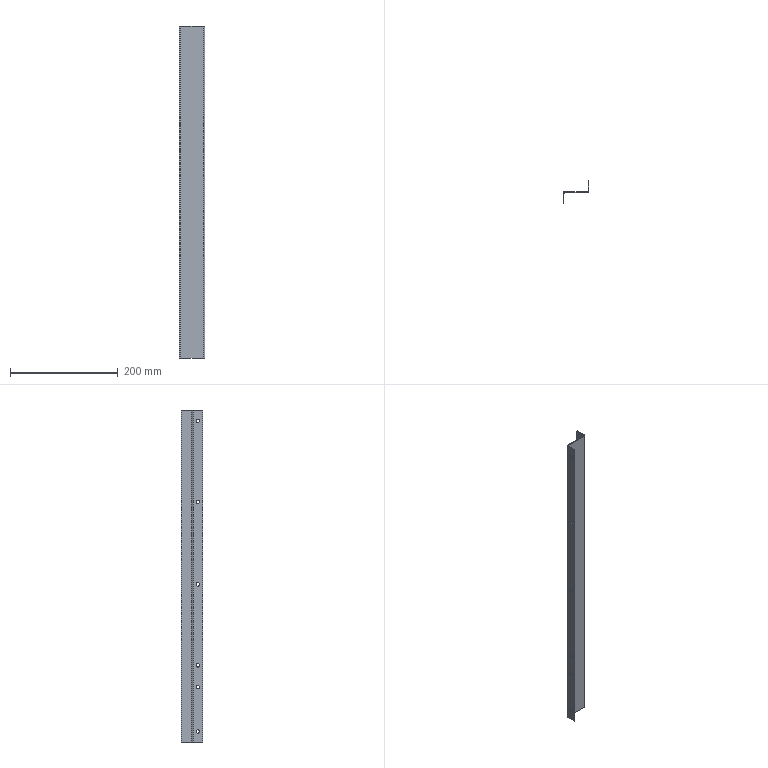Part | SolidWorks | features Cut 1, FlatPattern 1, SMBaseFlange 1, SheetMetal 1 | 1 solid | 34 faces | box 47.2 x 40 x 615 mm | volume 62089 mm3 | plane 18 | cylinder 16 | commonest cylinder face diameters 6.5 x12 2.4 x2 4.8 x2
STEP:
#1=CARTESIAN_POINT('',(1.2,12.25,595.));
#2=VERTEX_POINT('',#1);
#3=CARTESIAN_POINT('',(1.2,5.75,595.));
#4=VERTEX_POINT('',#3);
#5=CARTESIAN_POINT('',(1.2,9.,595.));
#6=DIRECTION('',(-1.,0.,0.));
#7=DIRECTION('',(0.,0.,1.));
#8=AXIS2_PLACEMENT_3D('',#5,#6,#7);
#9=CIRCLE('',#8,3.25);
#10=EDGE_CURVE('',#2,#4,#9,.T.);
#11=ORIENTED_EDGE('',*,*,#10,.F.);
#12=CARTESIAN_POINT('',(0.,12.25,595.));
#13=VERTEX_POINT('',#12);
#14=CARTESIAN_POINT('',(9.2,12.25,595.));
#15=DIRECTION('',(-1.,0.,0.));
#16=VECTOR('',#15,1000.);
#17=LINE('',#14,#16);
#18=EDGE_CURVE('',#2,#13,#17,.T.);
#19=ORIENTED_EDGE('',*,*,#18,.T.);
#20=CARTESIAN_POINT('',(0.,5.75,595.));
#21=VERTEX_POINT('',#20);
#22=CARTESIAN_POINT('',(0.,9.,595.));
#23=DIRECTION('',(-1.,0.,0.));
#24=DIRECTION('',(0.,0.,1.));
#25=AXIS2_PLACEMENT_3D('',#22,#23,#24);
#26=CIRCLE('',#25,3.25);
#27=EDGE_CURVE('',#13,#21,#26,.T.);
#28=ORIENTED_EDGE('',*,*,#27,.T.);
#29=CARTESIAN_POINT('',(9.2,5.75,595.));
#30=DIRECTION('',(-1.,0.,0.));
#31=VECTOR('',#30,1000.);
#32=LINE('',#29,#31);
#33=EDGE_CURVE('',#4,#21,#32,.T.);
#34=ORIENTED_EDGE('',*,*,#33,.F.);
#35=EDGE_LOOP('',(#11,#19,#28,#34));
#36=FACE_OUTER_BOUND('',#35,.T.);
#37=CARTESIAN_POINT('',(9.2,9.,595.));
#38=DIRECTION('',(-1.,0.,0.));
#39=DIRECTION('',(0.,-1.,0.));
#40=AXIS2_PLACEMENT_3D('',#37,#38,#39);
#41=CYLINDRICAL_SURFACE('',#40,3.25);
#42=ADVANCED_FACE('',(#36),#41,.F.);
#43=CARTESIAN_POINT('',(1.2,12.25,292.));
#44=VERTEX_POINT('',#43);
#45=CARTESIAN_POINT('',(1.2,5.75,292.));
#46=VERTEX_POINT('',#45);
#47=CARTESIAN_POINT('',(1.2,9.,292.));
#48=DIRECTION('',(-1.,0.,0.));
#49=DIRECTION('',(0.,0.,1.));
#50=AXIS2_PLACEMENT_3D('',#47,#48,#49);
#51=CIRCLE('',#50,3.25);
#52=EDGE_CURVE('',#44,#46,#51,.T.);
#53=ORIENTED_EDGE('',*,*,#52,.F.);
#54=CARTESIAN_POINT('',(0.,12.25,292.));
#55=VERTEX_POINT('',#54);
#56=CARTESIAN_POINT('',(9.2,12.25,292.));
#57=DIRECTION('',(-1.,0.,0.));
#58=VECTOR('',#57,1000.);
#59=LINE('',#56,#58);
#60=EDGE_CURVE('',#44,#55,#59,.T.);
#61=ORIENTED_EDGE('',*,*,#60,.T.);
#62=CARTESIAN_POINT('',(0.,5.75,292.));
#63=VERTEX_POINT('',#62);
#64=CARTESIAN_POINT('',(0.,9.,292.));
#65=DIRECTION('',(-1.,0.,0.));
#66=DIRECTION('',(0.,0.,1.));
#67=AXIS2_PLACEMENT_3D('',#64,#65,#66);
#68=CIRCLE('',#67,3.25);
#69=EDGE_CURVE('',#55,#63,#68,.T.);
#70=ORIENTED_EDGE('',*,*,#69,.T.);
#71=CARTESIAN_POINT('',(9.2,5.75,292.));
#72=DIRECTION('',(-1.,0.,0.));
#73=VECTOR('',#72,1000.);
#74=LINE('',#71,#73);
#75=EDGE_CURVE('',#46,#63,#74,.T.);
#76=ORIENTED_EDGE('',*,*,#75,.F.);
#77=EDGE_LOOP('',(#53,#61,#70,#76));
#78=FACE_OUTER_BOUND('',#77,.T.);
#79=CARTESIAN_POINT('',(9.2,9.,292.));
#80=DIRECTION('',(-1.,0.,0.));
#81=DIRECTION('',(0.,-1.,0.));
#82=AXIS2_PLACEMENT_3D('',#79,#80,#81);
#83=CYLINDRICAL_SURFACE('',#82,3.25);
#84=ADVANCED_FACE('',(#78),#83,.F.);
#85=CARTESIAN_POINT('',(1.2,12.25,445.));
#86=VERTEX_POINT('',#85);
#87=CARTESIAN_POINT('',(1.2,5.75,445.));
#88=VERTEX_POINT('',#87);
#89=CARTESIAN_POINT('',(1.2,9.,445.));
#90=DIRECTION('',(-1.,0.,0.));
#91=DIRECTION('',(0.,0.,1.));
#92=AXIS2_PLACEMENT_3D('',#89,#90,#91);
#93=CIRCLE('',#92,3.25);
#94=EDGE_CURVE('',#86,#88,#93,.T.);
#95=ORIENTED_EDGE('',*,*,#94,.F.);
#96=CARTESIAN_POINT('',(0.,12.25,445.));
#97=VERTEX_POINT('',#96);
#98=CARTESIAN_POINT('',(9.2,12.25,445.));
#99=DIRECTION('',(-1.,0.,0.));
#100=VECTOR('',#99,1000.);
#101=LINE('',#98,#100);
#102=EDGE_CURVE('',#86,#97,#101,.T.);
#103=ORIENTED_EDGE('',*,*,#102,.T.);
#104=CARTESIAN_POINT('',(0.,5.75,445.));
#105=VERTEX_POINT('',#104);
#106=CARTESIAN_POINT('',(0.,9.,445.));
#107=DIRECTION('',(-1.,0.,0.));
#108=DIRECTION('',(0.,0.,1.));
#109=AXIS2_PLACEMENT_3D('',#106,#107,#108);
#110=CIRCLE('',#109,3.25);
#111=EDGE_CURVE('',#97,#105,#110,.T.);
#112=ORIENTED_EDGE('',*,*,#111,.T.);
#113=CARTESIAN_POINT('',(9.2,5.75,445.));
#114=DIRECTION('',(-1.,0.,0.));
#115=VECTOR('',#114,1000.);
#116=LINE('',#113,#115);
#117=EDGE_CURVE('',#88,#105,#116,.T.);
#118=ORIENTED_EDGE('',*,*,#117,.F.);
#119=EDGE_LOOP('',(#95,#103,#112,#118));
#120=FACE_OUTER_BOUND('',#119,.T.);
#121=CARTESIAN_POINT('',(9.2,9.,445.));
#122=DIRECTION('',(-1.,0.,0.));
#123=DIRECTION('',(0.,-1.,0.));
#124=AXIS2_PLACEMENT_3D('',#121,#122,#123);
#125=CYLINDRICAL_SURFACE('',#124,3.25);
#126=ADVANCED_FACE('',(#120),#125,.F.);
#127=CARTESIAN_POINT('',(1.2,12.25,101.5));
#128=VERTEX_POINT('',#127);
#129=CARTESIAN_POINT('',(1.2,5.75,101.5));
#130=VERTEX_POINT('',#129);
#131=CARTESIAN_POINT('',(1.2,9.,101.5));
#132=DIRECTION('',(-1.,0.,0.));
#133=DIRECTION('',(0.,0.,1.));
#134=AXIS2_PLACEMENT_3D('',#131,#132,#133);
#135=CIRCLE('',#134,3.25);
#136=EDGE_CURVE('',#128,#130,#135,.T.);
#137=ORIENTED_EDGE('',*,*,#136,.F.);
#138=CARTESIAN_POINT('',(0.,12.25,101.5));
#139=VERTEX_POINT('',#138);
#140=CARTESIAN_POINT('',(9.2,12.25,101.5));
#141=DIRECTION('',(-1.,0.,0.));
#142=VECTOR('',#141,1000.);
#143=LINE('',#140,#142);
#144=EDGE_CURVE('',#128,#139,#143,.T.);
#145=ORIENTED_EDGE('',*,*,#144,.T.);
#146=CARTESIAN_POINT('',(0.,5.75,101.5));
#147=VERTEX_POINT('',#146);
#148=CARTESIAN_POINT('',(0.,9.,101.5));
#149=DIRECTION('',(-1.,0.,0.));
#150=DIRECTION('',(0.,0.,1.));
#151=AXIS2_PLACEMENT_3D('',#148,#149,#150);
#152=CIRCLE('',#151,3.25);
#153=EDGE_CURVE('',#139,#147,#152,.T.);
#154=ORIENTED_EDGE('',*,*,#153,.T.);
#155=CARTESIAN_POINT('',(9.2,5.75,101.5));
#156=DIRECTION('',(-1.,0.,0.));
#157=VECTOR('',#156,1000.);
#158=LINE('',#155,#157);
#159=EDGE_CURVE('',#130,#147,#158,.T.);
#160=ORIENTED_EDGE('',*,*,#159,.F.);
#161=EDGE_LOOP('',(#137,#145,#154,#160));
#162=FACE_OUTER_BOUND('',#161,.T.);
#163=CARTESIAN_POINT('',(9.2,9.,101.5));
#164=DIRECTION('',(-1.,0.,0.));
#165=DIRECTION('',(0.,-1.,0.));
#166=AXIS2_PLACEMENT_3D('',#163,#164,#165);
#167=CYLINDRICAL_SURFACE('',#166,3.25);
#168=ADVANCED_FACE('',(#162),#167,.F.);
#169=CARTESIAN_POINT('',(1.2,12.25,19.5));
#170=VERTEX_POINT('',#169);
#171=CARTESIAN_POINT('',(1.2,5.75,19.5));
#172=VERTEX_POINT('',#171);
#173=CARTESIAN_POINT('',(1.2,9.,19.5));
#174=DIRECTION('',(-1.,0.,0.));
#175=DIRECTION('',(0.,0.,1.));
#176=AXIS2_PLACEMENT_3D('',#173,#174,#175);
#177=CIRCLE('',#176,3.25);
#178=EDGE_CURVE('',#170,#172,#177,.T.);
#179=ORIENTED_EDGE('',*,*,#178,.F.);
#180=CARTESIAN_POINT('',(0.,12.25,19.5));
#181=VERTEX_POINT('',#180);
#182=CARTESIAN_POINT('',(9.2,12.25,19.5));
#183=DIRECTION('',(-1.,0.,0.));
#184=VECTOR('',#183,1000.);
#185=LINE('',#182,#184);
#186=EDGE_CURVE('',#170,#181,#185,.T.);
#187=ORIENTED_EDGE('',*,*,#186,.T.);
#188=CARTESIAN_POINT('',(0.,5.75,19.5));
#189=VERTEX_POINT('',#188);
#190=CARTESIAN_POINT('',(0.,9.,19.5));
#191=DIRECTION('',(-1.,0.,0.));
#192=DIRECTION('',(0.,0.,1.));
#193=AXIS2_PLACEMENT_3D('',#190,#191,#192);
#194=CIRCLE('',#193,3.25);
#195=EDGE_CURVE('',#181,#189,#194,.T.);
#196=ORIENTED_EDGE('',*,*,#195,.T.);
#197=CARTESIAN_POINT('',(9.2,5.75,19.5));
#198=DIRECTION('',(-1.,0.,0.));
#199=VECTOR('',#198,1000.);
#200=LINE('',#197,#199);
#201=EDGE_CURVE('',#172,#189,#200,.T.);
#202=ORIENTED_EDGE('',*,*,#201,.F.);
#203=EDGE_LOOP('',(#179,#187,#196,#202));
#204=FACE_OUTER_BOUND('',#203,.T.);
#205=CARTESIAN_POINT('',(9.2,9.,19.5));
#206=DIRECTION('',(-1.,0.,0.));
#207=DIRECTION('',(0.,-1.,0.));
#208=AXIS2_PLACEMENT_3D('',#205,#206,#207);
#209=CYLINDRICAL_SURFACE('',#208,3.25);
#210=ADVANCED_FACE('',(#204),#209,.F.);
#211=CARTESIAN_POINT('',(1.2,12.25,142.));
#212=VERTEX_POINT('',#211);
#213=CARTESIAN_POINT('',(1.2,5.75,142.));
#214=VERTEX_POINT('',#213);
#215=CARTESIAN_POINT('',(1.2,9.,142.));
#216=DIRECTION('',(-1.,0.,0.));
#217=DIRECTION('',(0.,0.,1.));
#218=AXIS2_PLACEMENT_3D('',#215,#216,#217);
#219=CIRCLE('',#218,3.25);
#220=EDGE_CURVE('',#212,#214,#219,.T.);
#221=ORIENTED_EDGE('',*,*,#220,.F.);
#222=CARTESIAN_POINT('',(0.,12.25,142.));
#223=VERTEX_POINT('',#222);
#224=CARTESIAN_POINT('',(9.2,12.25,142.));
#225=DIRECTION('',(-1.,0.,0.));
#226=VECTOR('',#225,1000.);
#227=LINE('',#224,#226);
#228=EDGE_CURVE('',#212,#223,#227,.T.);
#229=ORIENTED_EDGE('',*,*,#228,.T.);
#230=CARTESIAN_POINT('',(0.,5.75,142.));
#231=VERTEX_POINT('',#230);
#232=CARTESIAN_POINT('',(0.,9.,142.));
#233=DIRECTION('',(-1.,0.,0.));
#234=DIRECTION('',(0.,0.,1.));
#235=AXIS2_PLACEMENT_3D('',#232,#233,#234);
#236=CIRCLE('',#235,3.25);
#237=EDGE_CURVE('',#223,#231,#236,.T.);
#238=ORIENTED_EDGE('',*,*,#237,.T.);
#239=CARTESIAN_POINT('',(9.2,5.75,142.));
#240=DIRECTION('',(-1.,0.,0.));
#241=VECTOR('',#240,1000.);
#242=LINE('',#239,#241);
#243=EDGE_CURVE('',#214,#231,#242,.T.);
#244=ORIENTED_EDGE('',*,*,#243,.F.);
#245=EDGE_LOOP('',(#221,#229,#238,#244));
#246=FACE_OUTER_BOUND('',#245,.T.);
#247=CARTESIAN_POINT('',(9.2,9.,142.));
#248=DIRECTION('',(-1.,0.,0.));
#249=DIRECTION('',(0.,-1.,0.));
#250=AXIS2_PLACEMENT_3D('',#247,#248,#249);
#251=CYLINDRICAL_SURFACE('',#250,3.25);
#252=ADVANCED_FACE('',(#246),#251,.F.);
#253=CARTESIAN_POINT('',(2.4,20.,615.));
#254=VERTEX_POINT('',#253);
#255=CARTESIAN_POINT('',(2.4,18.8,615.));
#256=VERTEX_POINT('',#255);
#257=CARTESIAN_POINT('',(2.4,20.,615.));
#258=DIRECTION('',(0.,-1.,0.));
#259=VECTOR('',#258,1000.);
#260=LINE('',#257,#259);
#261=EDGE_CURVE('',#254,#256,#260,.T.);
#262=ORIENTED_EDGE('',*,*,#261,.F.);
#263=CARTESIAN_POINT('',(0.,17.6,615.));
#264=VERTEX_POINT('',#263);
#265=CARTESIAN_POINT('',(2.4,17.6,615.));
#266=DIRECTION('',(0.,0.,-1.));
#267=DIRECTION('',(1.,0.,0.));
#268=AXIS2_PLACEMENT_3D('',#265,#266,#267);
#269=CIRCLE('',#268,2.4);
#270=EDGE_CURVE('',#264,#254,#269,.T.);
#271=ORIENTED_EDGE('',*,*,#270,.F.);
#272=CARTESIAN_POINT('',(1.2,17.6,615.));
#273=VERTEX_POINT('',#272);
#274=CARTESIAN_POINT('',(1.2,17.6,615.));
#275=DIRECTION('',(-1.,0.,0.));
#276=VECTOR('',#275,1000.);
#277=LINE('',#274,#276);
#278=EDGE_CURVE('',#273,#264,#277,.T.);
#279=ORIENTED_EDGE('',*,*,#278,.F.);
#280=CARTESIAN_POINT('',(2.4,17.6,615.));
#281=DIRECTION('',(0.,0.,-1.));
#282=DIRECTION('',(1.,0.,0.));
#283=AXIS2_PLACEMENT_3D('',#280,#281,#282);
#284=CIRCLE('',#283,1.2);
#285=EDGE_CURVE('',#273,#256,#284,.T.);
#286=ORIENTED_EDGE('',*,*,#285,.T.);
#287=EDGE_LOOP('',(#262,#271,#279,#286));
#288=FACE_OUTER_BOUND('',#287,.T.);
#289=CARTESIAN_POINT('',(2.4,20.,615.));
#290=DIRECTION('',(0.,0.,1.));
#291=DIRECTION('',(1.,0.,0.));
#292=AXIS2_PLACEMENT_3D('',#289,#290,#291);
#293=PLANE('',#292);
#294=ADVANCED_FACE('',(#288),#293,.T.);
#295=CARTESIAN_POINT('',(44.8,20.,615.));
#296=VERTEX_POINT('',#295);
#297=CARTESIAN_POINT('',(0.,20.,615.));
#298=DIRECTION('',(1.,0.,0.));
#299=VECTOR('',#298,1000.);
#300=LINE('',#297,#299);
#301=EDGE_CURVE('',#254,#296,#300,.T.);
#302=ORIENTED_EDGE('',*,*,#301,.F.);
#303=ORIENTED_EDGE('',*,*,#261,.T.);
#304=CARTESIAN_POINT('',(44.8,18.8,615.));
#305=VERTEX_POINT('',#304);
#306=CARTESIAN_POINT('',(0.,18.8,615.));
#307=DIRECTION('',(1.,0.,0.));
#308=VECTOR('',#307,1000.);
#309=LINE('',#306,#308);
#310=EDGE_CURVE('',#256,#305,#309,.T.);
#311=ORIENTED_EDGE('',*,*,#310,.T.);
#312=CARTESIAN_POINT('',(44.8,18.8,615.));
#313=DIRECTION('',(0.,1.,0.));
#314=VECTOR('',#313,1000.);
#315=LINE('',#312,#314);
#316=EDGE_CURVE('',#305,#296,#315,.T.);
#317=ORIENTED_EDGE('',*,*,#316,.T.);
#318=EDGE_LOOP('',(#302,#303,#311,#317));
#319=FACE_OUTER_BOUND('',#318,.T.);
#320=CARTESIAN_POINT('',(1.2,17.6,615.));
#321=DIRECTION('',(0.,0.,1.));
#322=DIRECTION('',(1.,0.,0.));
#323=AXIS2_PLACEMENT_3D('',#320,#321,#322);
#324=PLANE('',#323);
#325=ADVANCED_FACE('',(#319),#324,.T.);
#326=CARTESIAN_POINT('',(0.,17.6,0.));
#327=VERTEX_POINT('',#326);
#328=CARTESIAN_POINT('',(1.2,17.6,0.));
#329=VERTEX_POINT('',#328);
#330=CARTESIAN_POINT('',(0.,17.6,0.));
#331=DIRECTION('',(1.,0.,0.));
#332=VECTOR('',#331,1000.);
#333=LINE('',#330,#332);
#334=EDGE_CURVE('',#327,#329,#333,.T.);
#335=ORIENTED_EDGE('',*,*,#334,.F.);
#336=CARTESIAN_POINT('',(2.4,20.,0.));
#337=VERTEX_POINT('',#336);
#338=CARTESIAN_POINT('',(2.4,17.6,0.));
#339=DIRECTION('',(0.,0.,-1.));
#340=DIRECTION('',(1.,0.,0.));
#341=AXIS2_PLACEMENT_3D('',#338,#339,#340);
#342=CIRCLE('',#341,2.4);
#343=EDGE_CURVE('',#327,#337,#342,.T.);
#344=ORIENTED_EDGE('',*,*,#343,.T.);
#345=CARTESIAN_POINT('',(2.4,18.8,0.));
#346=VERTEX_POINT('',#345);
#347=CARTESIAN_POINT('',(2.4,18.8,0.));
#348=DIRECTION('',(0.,1.,0.));
#349=VECTOR('',#348,1000.);
#350=LINE('',#347,#349);
#351=EDGE_CURVE('',#346,#337,#350,.T.);
#352=ORIENTED_EDGE('',*,*,#351,.F.);
#353=CARTESIAN_POINT('',(2.4,17.6,0.));
#354=DIRECTION('',(0.,0.,-1.));
#355=DIRECTION('',(1.,0.,0.));
#356=AXIS2_PLACEMENT_3D('',#353,#354,#355);
#357=CIRCLE('',#356,1.2);
#358=EDGE_CURVE('',#329,#346,#357,.T.);
#359=ORIENTED_EDGE('',*,*,#358,.F.);
#360=EDGE_LOOP('',(#335,#344,#352,#359));
#361=FACE_OUTER_BOUND('',#360,.T.);
#362=CARTESIAN_POINT('',(0.,17.6,0.));
#363=DIRECTION('',(0.,0.,-1.));
#364=DIRECTION('',(-1.,0.,0.));
#365=AXIS2_PLACEMENT_3D('',#362,#363,#364);
#366=PLANE('',#365);
#367=ADVANCED_FACE('',(#361),#366,.T.);
#368=CARTESIAN_POINT('',(0.,0.,0.));
#369=VERTEX_POINT('',#368);
#370=CARTESIAN_POINT('',(0.,0.,0.));
#371=DIRECTION('',(0.,1.,0.));
#372=VECTOR('',#371,1000.);
#373=LINE('',#370,#372);
#374=EDGE_CURVE('',#369,#327,#373,.T.);
#375=ORIENTED_EDGE('',*,*,#374,.T.);
#376=ORIENTED_EDGE('',*,*,#334,.T.);
#377=CARTESIAN_POINT('',(1.2,0.,0.));
#378=VERTEX_POINT('',#377);
#379=CARTESIAN_POINT('',(1.2,0.,0.));
#380=DIRECTION('',(0.,1.,0.));
#381=VECTOR('',#380,1000.);
#382=LINE('',#379,#381);
#383=EDGE_CURVE('',#378,#329,#382,.T.);
#384=ORIENTED_EDGE('',*,*,#383,.F.);
#385=CARTESIAN_POINT('',(1.2,0.,0.));
#386=DIRECTION('',(-1.,0.,0.));
#387=VECTOR('',#386,1000.);
#388=LINE('',#385,#387);
#389=EDGE_CURVE('',#378,#369,#388,.T.);
#390=ORIENTED_EDGE('',*,*,#389,.T.);
#391=EDGE_LOOP('',(#375,#376,#384,#390));
#392=FACE_OUTER_BOUND('',#391,.T.);
#393=CARTESIAN_POINT('',(2.4,18.8,0.));
#394=DIRECTION('',(0.,0.,-1.));
#395=DIRECTION('',(-1.,0.,0.));
#396=AXIS2_PLACEMENT_3D('',#393,#394,#395);
#397=PLANE('',#396);
#398=ADVANCED_FACE('',(#392),#397,.T.);
#399=CARTESIAN_POINT('',(46.,21.2,615.));
#400=VERTEX_POINT('',#399);
#401=CARTESIAN_POINT('',(47.2,21.2,615.));
#402=VERTEX_POINT('',#401);
#403=CARTESIAN_POINT('',(46.,21.2,615.));
#404=DIRECTION('',(1.,0.,0.));
#405=VECTOR('',#404,1000.);
#406=LINE('',#403,#405);
#407=EDGE_CURVE('',#400,#402,#406,.T.);
#408=ORIENTED_EDGE('',*,*,#407,.F.);
#409=CARTESIAN_POINT('',(44.8,21.2,615.));
#410=DIRECTION('',(0.,0.,1.));
#411=DIRECTION('',(-1.,0.,0.));
#412=AXIS2_PLACEMENT_3D('',#409,#410,#411);
#413=CIRCLE('',#412,1.2);
#414=EDGE_CURVE('',#296,#400,#413,.T.);
#415=ORIENTED_EDGE('',*,*,#414,.F.);
#416=ORIENTED_EDGE('',*,*,#316,.F.);
#417=CARTESIAN_POINT('',(44.8,21.2,615.));
#418=DIRECTION('',(0.,0.,1.));
#419=DIRECTION('',(1.,0.,0.));
#420=AXIS2_PLACEMENT_3D('',#417,#418,#419);
#421=CIRCLE('',#420,2.4);
#422=EDGE_CURVE('',#305,#402,#421,.T.);
#423=ORIENTED_EDGE('',*,*,#422,.T.);
#424=EDGE_LOOP('',(#408,#415,#416,#423));
#425=FACE_OUTER_BOUND('',#424,.T.);
#426=CARTESIAN_POINT('',(46.,21.2,615.));
#427=DIRECTION('',(0.,0.,1.));
#428=DIRECTION('',(1.,0.,0.));
#429=AXIS2_PLACEMENT_3D('',#426,#427,#428);
#430=PLANE('',#429);
#431=ADVANCED_FACE('',(#425),#430,.T.);
#432=CARTESIAN_POINT('',(46.,40.,615.));
#433=VERTEX_POINT('',#432);
#434=CARTESIAN_POINT('',(46.,20.,615.));
#435=DIRECTION('',(0.,1.,0.));
#436=VECTOR('',#435,1000.);
#437=LINE('',#434,#436);
#438=EDGE_CURVE('',#400,#433,#437,.T.);
#439=ORIENTED_EDGE('',*,*,#438,.F.);
#440=ORIENTED_EDGE('',*,*,#407,.T.);
#441=CARTESIAN_POINT('',(47.2,40.,615.));
#442=VERTEX_POINT('',#441);
#443=CARTESIAN_POINT('',(47.2,20.,615.));
#444=DIRECTION('',(0.,1.,0.));
#445=VECTOR('',#444,1000.);
#446=LINE('',#443,#445);
#447=EDGE_CURVE('',#402,#442,#446,.T.);
#448=ORIENTED_EDGE('',*,*,#447,.T.);
#449=CARTESIAN_POINT('',(46.,40.,615.));
#450=DIRECTION('',(1.,0.,0.));
#451=VECTOR('',#450,1000.);
#452=LINE('',#449,#451);
#453=EDGE_CURVE('',#433,#442,#452,.T.);
#454=ORIENTED_EDGE('',*,*,#453,.F.);
#455=EDGE_LOOP('',(#439,#440,#448,#454));
#456=FACE_OUTER_BOUND('',#455,.T.);
#457=CARTESIAN_POINT('',(44.8,18.8,615.));
#458=DIRECTION('',(0.,0.,1.));
#459=DIRECTION('',(1.,0.,0.));
#460=AXIS2_PLACEMENT_3D('',#457,#458,#459);
#461=PLANE('',#460);
#462=ADVANCED_FACE('',(#456),#461,.T.);
#463=CARTESIAN_POINT('',(44.8,20.,0.));
#464=VERTEX_POINT('',#463);
#465=CARTESIAN_POINT('',(44.8,18.8,0.));
#466=VERTEX_POINT('',#465);
#467=CARTESIAN_POINT('',(44.8,20.,0.));
#468=DIRECTION('',(0.,-1.,0.));
#469=VECTOR('',#468,1000.);
#470=LINE('',#467,#469);
#471=EDGE_CURVE('',#464,#466,#470,.T.);
#472=ORIENTED_EDGE('',*,*,#471,.F.);
#473=CARTESIAN_POINT('',(46.,21.2,0.));
#474=VERTEX_POINT('',#473);
#475=CARTESIAN_POINT('',(44.8,21.2,0.));
#476=DIRECTION('',(0.,0.,1.));
#477=DIRECTION('',(-1.,0.,0.));
#478=AXIS2_PLACEMENT_3D('',#475,#476,#477);
#479=CIRCLE('',#478,1.2);
#480=EDGE_CURVE('',#464,#474,#479,.T.);
#481=ORIENTED_EDGE('',*,*,#480,.T.);
#482=CARTESIAN_POINT('',(47.2,21.2,0.));
#483=VERTEX_POINT('',#482);
#484=CARTESIAN_POINT('',(47.2,21.2,0.));
#485=DIRECTION('',(-1.,0.,0.));
#486=VECTOR('',#485,1000.);
#487=LINE('',#484,#486);
#488=EDGE_CURVE('',#483,#474,#487,.T.);
#489=ORIENTED_EDGE('',*,*,#488,.F.);
#490=CARTESIAN_POINT('',(44.8,21.2,0.));
#491=DIRECTION('',(0.,0.,1.));
#492=DIRECTION('',(1.,0.,0.));
#493=AXIS2_PLACEMENT_3D('',#490,#491,#492);
#494=CIRCLE('',#493,2.4);
#495=EDGE_CURVE('',#466,#483,#494,.T.);
#496=ORIENTED_EDGE('',*,*,#495,.F.);
#497=EDGE_LOOP('',(#472,#481,#489,#496));
#498=FACE_OUTER_BOUND('',#497,.T.);
#499=CARTESIAN_POINT('',(44.8,20.,0.));
#500=DIRECTION('',(0.,0.,-1.));
#501=DIRECTION('',(-1.,0.,0.));
#502=AXIS2_PLACEMENT_3D('',#499,#500,#501);
#503=PLANE('',#502);
#504=ADVANCED_FACE('',(#498),#503,.T.);
#505=CARTESIAN_POINT('',(0.,20.,0.));
#506=DIRECTION('',(1.,0.,0.));
#507=VECTOR('',#506,1000.);
#508=LINE('',#505,#507);
#509=EDGE_CURVE('',#337,#464,#508,.T.);
#510=ORIENTED_EDGE('',*,*,#509,.T.);
#511=ORIENTED_EDGE('',*,*,#471,.T.);
#512=CARTESIAN_POINT('',(0.,18.8,0.));
#513=DIRECTION('',(1.,0.,0.));
#514=VECTOR('',#513,1000.);
#515=LINE('',#512,#514);
#516=EDGE_CURVE('',#346,#466,#515,.T.);
#517=ORIENTED_EDGE('',*,*,#516,.F.);
#518=ORIENTED_EDGE('',*,*,#351,.T.);
#519=EDGE_LOOP('',(#510,#511,#517,#518));
#520=FACE_OUTER_BOUND('',#519,.T.);
#521=CARTESIAN_POINT('',(47.2,21.2,0.));
#522=DIRECTION('',(0.,0.,-1.));
#523=DIRECTION('',(-1.,0.,0.));
#524=AXIS2_PLACEMENT_3D('',#521,#522,#523);
#525=PLANE('',#524);
#526=ADVANCED_FACE('',(#520),#525,.T.);
#527=CARTESIAN_POINT('',(47.2,40.,0.));
#528=VERTEX_POINT('',#527);
#529=CARTESIAN_POINT('',(47.2,20.,0.));
#530=DIRECTION('',(0.,1.,0.));
#531=VECTOR('',#530,1000.);
#532=LINE('',#529,#531);
#533=EDGE_CURVE('',#483,#528,#532,.T.);
#534=ORIENTED_EDGE('',*,*,#533,.T.);
#535=CARTESIAN_POINT('',(47.2,40.,615.));
#536=DIRECTION('',(0.,0.,-1.));
#537=VECTOR('',#536,1000.);
#538=LINE('',#535,#537);
#539=EDGE_CURVE('',#442,#528,#538,.T.);
#540=ORIENTED_EDGE('',*,*,#539,.F.);
#541=ORIENTED_EDGE('',*,*,#447,.F.);
#542=CARTESIAN_POINT('',(47.2,21.2,615.));
#543=DIRECTION('',(0.,0.,-1.));
#544=VECTOR('',#543,1000.);
#545=LINE('',#542,#544);
#546=EDGE_CURVE('',#402,#483,#545,.T.);
#547=ORIENTED_EDGE('',*,*,#546,.T.);
#548=EDGE_LOOP('',(#534,#540,#541,#547));
#549=FACE_OUTER_BOUND('',#548,.T.);
#550=CARTESIAN_POINT('',(47.2,20.,615.));
#551=DIRECTION('',(-1.,0.,0.));
#552=DIRECTION('',(0.,0.,1.));
#553=AXIS2_PLACEMENT_3D('',#550,#551,#552);
#554=PLANE('',#553);
#555=ADVANCED_FACE('',(#549),#554,.F.);
#556=CARTESIAN_POINT('',(46.,40.,0.));
#557=VERTEX_POINT('',#556);
#558=CARTESIAN_POINT('',(46.,40.,0.));
#559=DIRECTION('',(1.,0.,0.));
#560=VECTOR('',#559,1000.);
#561=LINE('',#558,#560);
#562=EDGE_CURVE('',#557,#528,#561,.T.);
#563=ORIENTED_EDGE('',*,*,#562,.F.);
#564=CARTESIAN_POINT('',(46.,40.,615.));
#565=DIRECTION('',(0.,0.,-1.));
#566=VECTOR('',#565,1000.);
#567=LINE('',#564,#566);
#568=EDGE_CURVE('',#433,#557,#567,.T.);
#569=ORIENTED_EDGE('',*,*,#568,.F.);
#570=ORIENTED_EDGE('',*,*,#453,.T.);
#571=ORIENTED_EDGE('',*,*,#539,.T.);
#572=EDGE_LOOP('',(#563,#569,#570,#571));
#573=FACE_OUTER_BOUND('',#572,.T.);
#574=CARTESIAN_POINT('',(46.,40.,615.));
#575=DIRECTION('',(0.,1.,0.));
#576=DIRECTION('',(0.,0.,1.));
#577=AXIS2_PLACEMENT_3D('',#574,#575,#576);
#578=PLANE('',#577);
#579=ADVANCED_FACE('',(#573),#578,.T.);
#580=CARTESIAN_POINT('',(46.,20.,0.));
#581=DIRECTION('',(0.,1.,0.));
#582=VECTOR('',#581,1000.);
#583=LINE('',#580,#582);
#584=EDGE_CURVE('',#474,#557,#583,.T.);
#585=ORIENTED_EDGE('',*,*,#584,.F.);
#586=CARTESIAN_POINT('',(46.,21.2,615.));
#587=DIRECTION('',(0.,0.,-1.));
#588=VECTOR('',#587,1000.);
#589=LINE('',#586,#588);
#590=EDGE_CURVE('',#400,#474,#589,.T.);
#591=ORIENTED_EDGE('',*,*,#590,.F.);
#592=ORIENTED_EDGE('',*,*,#438,.T.);
#593=ORIENTED_EDGE('',*,*,#568,.T.);
#594=EDGE_LOOP('',(#585,#591,#592,#593));
#595=FACE_OUTER_BOUND('',#594,.T.);
#596=CARTESIAN_POINT('',(46.,20.,615.));
#597=DIRECTION('',(-1.,0.,0.));
#598=DIRECTION('',(0.,0.,1.));
#599=AXIS2_PLACEMENT_3D('',#596,#597,#598);
#600=PLANE('',#599);
#601=ADVANCED_FACE('',(#595),#600,.T.);
#602=ORIENTED_EDGE('',*,*,#480,.F.);
#603=CARTESIAN_POINT('',(44.8,20.,615.));
#604=DIRECTION('',(0.,0.,-1.));
#605=VECTOR('',#604,1000.);
#606=LINE('',#603,#605);
#607=EDGE_CURVE('',#296,#464,#606,.T.);
#608=ORIENTED_EDGE('',*,*,#607,.F.);
#609=ORIENTED_EDGE('',*,*,#414,.T.);
#610=ORIENTED_EDGE('',*,*,#590,.T.);
#611=EDGE_LOOP('',(#602,#608,#609,#610));
#612=FACE_OUTER_BOUND('',#611,.T.);
#613=CARTESIAN_POINT('',(44.8,21.2,615.));
#614=DIRECTION('',(0.,0.,-1.));
#615=DIRECTION('',(-1.,0.,0.));
#616=AXIS2_PLACEMENT_3D('',#613,#614,#615);
#617=CYLINDRICAL_SURFACE('',#616,1.2);
#618=ADVANCED_FACE('',(#612),#617,.F.);
#619=ORIENTED_EDGE('',*,*,#509,.F.);
#620=CARTESIAN_POINT('',(2.4,20.,615.));
#621=DIRECTION('',(0.,0.,-1.));
#622=VECTOR('',#621,1000.);
#623=LINE('',#620,#622);
#624=EDGE_CURVE('',#254,#337,#623,.T.);
#625=ORIENTED_EDGE('',*,*,#624,.F.);
#626=ORIENTED_EDGE('',*,*,#301,.T.);
#627=ORIENTED_EDGE('',*,*,#607,.T.);
#628=EDGE_LOOP('',(#619,#625,#626,#627));
#629=FACE_OUTER_BOUND('',#628,.T.);
#630=CARTESIAN_POINT('',(0.,20.,615.));
#631=DIRECTION('',(0.,1.,0.));
#632=DIRECTION('',(0.,0.,1.));
#633=AXIS2_PLACEMENT_3D('',#630,#631,#632);
#634=PLANE('',#633);
#635=ADVANCED_FACE('',(#629),#634,.T.);
#636=ORIENTED_EDGE('',*,*,#343,.F.);
#637=CARTESIAN_POINT('',(0.,17.6,615.));
#638=DIRECTION('',(0.,0.,-1.));
#639=VECTOR('',#638,1000.);
#640=LINE('',#637,#639);
#641=EDGE_CURVE('',#264,#327,#640,.T.);
#642=ORIENTED_EDGE('',*,*,#641,.F.);
#643=ORIENTED_EDGE('',*,*,#270,.T.);
#644=ORIENTED_EDGE('',*,*,#624,.T.);
#645=EDGE_LOOP('',(#636,#642,#643,#644));
#646=FACE_OUTER_BOUND('',#645,.T.);
#647=CARTESIAN_POINT('',(2.4,17.6,615.));
#648=DIRECTION('',(0.,0.,-1.));
#649=DIRECTION('',(-1.,0.,0.));
#650=AXIS2_PLACEMENT_3D('',#647,#648,#649);
#651=CYLINDRICAL_SURFACE('',#650,2.4);
#652=ADVANCED_FACE('',(#646),#651,.T.);
#653=CARTESIAN_POINT('',(0.,9.,595.));
#654=DIRECTION('',(-1.,0.,0.));
#655=DIRECTION('',(0.,0.,1.));
#656=AXIS2_PLACEMENT_3D('',#653,#654,#655);
#657=CIRCLE('',#656,3.25);
#658=EDGE_CURVE('',#21,#13,#657,.T.);
#659=ORIENTED_EDGE('',*,*,#658,.F.);
#660=ORIENTED_EDGE('',*,*,#27,.F.);
#661=EDGE_LOOP('',(#659,#660));
#662=FACE_BOUND('',#661,.T.);
#663=CARTESIAN_POINT('',(0.,9.,292.));
#664=DIRECTION('',(-1.,0.,0.));
#665=DIRECTION('',(0.,0.,1.));
#666=AXIS2_PLACEMENT_3D('',#663,#664,#665);
#667=CIRCLE('',#666,3.25);
#668=EDGE_CURVE('',#63,#55,#667,.T.);
#669=ORIENTED_EDGE('',*,*,#668,.F.);
#670=ORIENTED_EDGE('',*,*,#69,.F.);
#671=EDGE_LOOP('',(#669,#670));
#672=FACE_BOUND('',#671,.T.);
#673=CARTESIAN_POINT('',(0.,9.,445.));
#674=DIRECTION('',(-1.,0.,0.));
#675=DIRECTION('',(0.,0.,1.));
#676=AXIS2_PLACEMENT_3D('',#673,#674,#675);
#677=CIRCLE('',#676,3.25);
#678=EDGE_CURVE('',#105,#97,#677,.T.);
#679=ORIENTED_EDGE('',*,*,#678,.F.);
#680=ORIENTED_EDGE('',*,*,#111,.F.);
#681=EDGE_LOOP('',(#679,#680));
#682=FACE_BOUND('',#681,.T.);
#683=CARTESIAN_POINT('',(0.,9.,101.5));
#684=DIRECTION('',(-1.,0.,0.));
#685=DIRECTION('',(0.,0.,1.));
#686=AXIS2_PLACEMENT_3D('',#683,#684,#685);
#687=CIRCLE('',#686,3.25);
#688=EDGE_CURVE('',#147,#139,#687,.T.);
#689=ORIENTED_EDGE('',*,*,#688,.F.);
#690=ORIENTED_EDGE('',*,*,#153,.F.);
#691=EDGE_LOOP('',(#689,#690));
#692=FACE_BOUND('',#691,.T.);
#693=CARTESIAN_POINT('',(0.,9.,19.5));
#694=DIRECTION('',(-1.,0.,0.));
#695=DIRECTION('',(0.,0.,1.));
#696=AXIS2_PLACEMENT_3D('',#693,#694,#695);
#697=CIRCLE('',#696,3.25);
#698=EDGE_CURVE('',#189,#181,#697,.T.);
#699=ORIENTED_EDGE('',*,*,#698,.F.);
#700=ORIENTED_EDGE('',*,*,#195,.F.);
#701=EDGE_LOOP('',(#699,#700));
#702=FACE_BOUND('',#701,.T.);
#703=CARTESIAN_POINT('',(0.,9.,142.));
#704=DIRECTION('',(-1.,0.,0.));
#705=DIRECTION('',(0.,0.,1.));
#706=AXIS2_PLACEMENT_3D('',#703,#704,#705);
#707=CIRCLE('',#706,3.25);
#708=EDGE_CURVE('',#231,#223,#707,.T.);
#709=ORIENTED_EDGE('',*,*,#708,.F.);
#710=ORIENTED_EDGE('',*,*,#237,.F.);
#711=EDGE_LOOP('',(#709,#710));
#712=FACE_BOUND('',#711,.T.);
#713=ORIENTED_EDGE('',*,*,#374,.F.);
#714=CARTESIAN_POINT('',(0.,0.,615.));
#715=VERTEX_POINT('',#714);
#716=CARTESIAN_POINT('',(0.,0.,615.));
#717=DIRECTION('',(0.,0.,-1.));
#718=VECTOR('',#717,1000.);
#719=LINE('',#716,#718);
#720=EDGE_CURVE('',#715,#369,#719,.T.);
#721=ORIENTED_EDGE('',*,*,#720,.F.);
#722=CARTESIAN_POINT('',(0.,0.,615.));
#723=DIRECTION('',(0.,1.,0.));
#724=VECTOR('',#723,1000.);
#725=LINE('',#722,#724);
#726=EDGE_CURVE('',#715,#264,#725,.T.);
#727=ORIENTED_EDGE('',*,*,#726,.T.);
#728=ORIENTED_EDGE('',*,*,#641,.T.);
#729=EDGE_LOOP('',(#713,#721,#727,#728));
#730=FACE_OUTER_BOUND('',#729,.T.);
#731=CARTESIAN_POINT('',(0.,0.,615.));
#732=DIRECTION('',(-1.,0.,0.));
#733=DIRECTION('',(0.,0.,1.));
#734=AXIS2_PLACEMENT_3D('',#731,#732,#733);
#735=PLANE('',#734);
#736=ADVANCED_FACE('',(#662,#672,#682,#692,#702,#712,#730),#735,.T.);
#737=ORIENTED_EDGE('',*,*,#389,.F.);
#738=CARTESIAN_POINT('',(1.2,0.,615.));
#739=VERTEX_POINT('',#738);
#740=CARTESIAN_POINT('',(1.2,0.,615.));
#741=DIRECTION('',(0.,0.,-1.));
#742=VECTOR('',#741,1000.);
#743=LINE('',#740,#742);
#744=EDGE_CURVE('',#739,#378,#743,.T.);
#745=ORIENTED_EDGE('',*,*,#744,.F.);
#746=CARTESIAN_POINT('',(1.2,0.,615.));
#747=DIRECTION('',(-1.,0.,0.));
#748=VECTOR('',#747,1000.);
#749=LINE('',#746,#748);
#750=EDGE_CURVE('',#739,#715,#749,.T.);
#751=ORIENTED_EDGE('',*,*,#750,.T.);
#752=ORIENTED_EDGE('',*,*,#720,.T.);
#753=EDGE_LOOP('',(#737,#745,#751,#752));
#754=FACE_OUTER_BOUND('',#753,.T.);
#755=CARTESIAN_POINT('',(1.2,0.,615.));
#756=DIRECTION('',(0.,-1.,0.));
#757=DIRECTION('',(0.,0.,-1.));
#758=AXIS2_PLACEMENT_3D('',#755,#756,#757);
#759=PLANE('',#758);
#760=ADVANCED_FACE('',(#754),#759,.T.);
#761=CARTESIAN_POINT('',(1.2,9.,595.));
#762=DIRECTION('',(-1.,0.,0.));
#763=DIRECTION('',(0.,0.,1.));
#764=AXIS2_PLACEMENT_3D('',#761,#762,#763);
#765=CIRCLE('',#764,3.25);
#766=EDGE_CURVE('',#4,#2,#765,.T.);
#767=ORIENTED_EDGE('',*,*,#766,.T.);
#768=ORIENTED_EDGE('',*,*,#10,.T.);
#769=EDGE_LOOP('',(#767,#768));
#770=FACE_BOUND('',#769,.T.);
#771=CARTESIAN_POINT('',(1.2,9.,292.));
#772=DIRECTION('',(-1.,0.,0.));
#773=DIRECTION('',(0.,0.,1.));
#774=AXIS2_PLACEMENT_3D('',#771,#772,#773);
#775=CIRCLE('',#774,3.25);
#776=EDGE_CURVE('',#46,#44,#775,.T.);
#777=ORIENTED_EDGE('',*,*,#776,.T.);
#778=ORIENTED_EDGE('',*,*,#52,.T.);
#779=EDGE_LOOP('',(#777,#778));
#780=FACE_BOUND('',#779,.T.);
#781=CARTESIAN_POINT('',(1.2,9.,445.));
#782=DIRECTION('',(-1.,0.,0.));
#783=DIRECTION('',(0.,0.,1.));
#784=AXIS2_PLACEMENT_3D('',#781,#782,#783);
#785=CIRCLE('',#784,3.25);
#786=EDGE_CURVE('',#88,#86,#785,.T.);
#787=ORIENTED_EDGE('',*,*,#786,.T.);
#788=ORIENTED_EDGE('',*,*,#94,.T.);
#789=EDGE_LOOP('',(#787,#788));
#790=FACE_BOUND('',#789,.T.);
#791=CARTESIAN_POINT('',(1.2,9.,101.5));
#792=DIRECTION('',(-1.,0.,0.));
#793=DIRECTION('',(0.,0.,1.));
#794=AXIS2_PLACEMENT_3D('',#791,#792,#793);
#795=CIRCLE('',#794,3.25);
#796=EDGE_CURVE('',#130,#128,#795,.T.);
#797=ORIENTED_EDGE('',*,*,#796,.T.);
#798=ORIENTED_EDGE('',*,*,#136,.T.);
#799=EDGE_LOOP('',(#797,#798));
#800=FACE_BOUND('',#799,.T.);
#801=CARTESIAN_POINT('',(1.2,9.,19.5));
#802=DIRECTION('',(-1.,0.,0.));
#803=DIRECTION('',(0.,0.,1.));
#804=AXIS2_PLACEMENT_3D('',#801,#802,#803);
#805=CIRCLE('',#804,3.25);
#806=EDGE_CURVE('',#172,#170,#805,.T.);
#807=ORIENTED_EDGE('',*,*,#806,.T.);
#808=ORIENTED_EDGE('',*,*,#178,.T.);
#809=EDGE_LOOP('',(#807,#808));
#810=FACE_BOUND('',#809,.T.);
#811=CARTESIAN_POINT('',(1.2,9.,142.));
#812=DIRECTION('',(-1.,0.,0.));
#813=DIRECTION('',(0.,0.,1.));
#814=AXIS2_PLACEMENT_3D('',#811,#812,#813);
#815=CIRCLE('',#814,3.25);
#816=EDGE_CURVE('',#214,#212,#815,.T.);
#817=ORIENTED_EDGE('',*,*,#816,.T.);
#818=ORIENTED_EDGE('',*,*,#220,.T.);
#819=EDGE_LOOP('',(#817,#818));
#820=FACE_BOUND('',#819,.T.);
#821=ORIENTED_EDGE('',*,*,#383,.T.);
#822=CARTESIAN_POINT('',(1.2,17.6,615.));
#823=DIRECTION('',(0.,0.,-1.));
#824=VECTOR('',#823,1000.);
#825=LINE('',#822,#824);
#826=EDGE_CURVE('',#273,#329,#825,.T.);
#827=ORIENTED_EDGE('',*,*,#826,.F.);
#828=CARTESIAN_POINT('',(1.2,0.,615.));
#829=DIRECTION('',(0.,1.,0.));
#830=VECTOR('',#829,1000.);
#831=LINE('',#828,#830);
#832=EDGE_CURVE('',#739,#273,#831,.T.);
#833=ORIENTED_EDGE('',*,*,#832,.F.);
#834=ORIENTED_EDGE('',*,*,#744,.T.);
#835=EDGE_LOOP('',(#821,#827,#833,#834));
#836=FACE_OUTER_BOUND('',#835,.T.);
#837=CARTESIAN_POINT('',(1.2,0.,615.));
#838=DIRECTION('',(-1.,0.,0.));
#839=DIRECTION('',(0.,0.,1.));
#840=AXIS2_PLACEMENT_3D('',#837,#838,#839);
#841=PLANE('',#840);
#842=ADVANCED_FACE('',(#770,#780,#790,#800,#810,#820,#836),#841,.F.);
#843=ORIENTED_EDGE('',*,*,#358,.T.);
#844=CARTESIAN_POINT('',(2.4,18.8,615.));
#845=DIRECTION('',(0.,0.,-1.));
#846=VECTOR('',#845,1000.);
#847=LINE('',#844,#846);
#848=EDGE_CURVE('',#256,#346,#847,.T.);
#849=ORIENTED_EDGE('',*,*,#848,.F.);
#850=ORIENTED_EDGE('',*,*,#285,.F.);
#851=ORIENTED_EDGE('',*,*,#826,.T.);
#852=EDGE_LOOP('',(#843,#849,#850,#851));
#853=FACE_OUTER_BOUND('',#852,.T.);
#854=CARTESIAN_POINT('',(2.4,17.6,615.));
#855=DIRECTION('',(0.,0.,-1.));
#856=DIRECTION('',(-1.,0.,0.));
#857=AXIS2_PLACEMENT_3D('',#854,#855,#856);
#858=CYLINDRICAL_SURFACE('',#857,1.2);
#859=ADVANCED_FACE('',(#853),#858,.F.);
#860=ORIENTED_EDGE('',*,*,#516,.T.);
#861=CARTESIAN_POINT('',(44.8,18.8,615.));
#862=DIRECTION('',(0.,0.,-1.));
#863=VECTOR('',#862,1000.);
#864=LINE('',#861,#863);
#865=EDGE_CURVE('',#305,#466,#864,.T.);
#866=ORIENTED_EDGE('',*,*,#865,.F.);
#867=ORIENTED_EDGE('',*,*,#310,.F.);
#868=ORIENTED_EDGE('',*,*,#848,.T.);
#869=EDGE_LOOP('',(#860,#866,#867,#868));
#870=FACE_OUTER_BOUND('',#869,.T.);
#871=CARTESIAN_POINT('',(0.,18.8,615.));
#872=DIRECTION('',(0.,1.,0.));
#873=DIRECTION('',(0.,0.,1.));
#874=AXIS2_PLACEMENT_3D('',#871,#872,#873);
#875=PLANE('',#874);
#876=ADVANCED_FACE('',(#870),#875,.F.);
#877=ORIENTED_EDGE('',*,*,#495,.T.);
#878=ORIENTED_EDGE('',*,*,#546,.F.);
#879=ORIENTED_EDGE('',*,*,#422,.F.);
#880=ORIENTED_EDGE('',*,*,#865,.T.);
#881=EDGE_LOOP('',(#877,#878,#879,#880));
#882=FACE_OUTER_BOUND('',#881,.T.);
#883=CARTESIAN_POINT('',(44.8,21.2,615.));
#884=DIRECTION('',(0.,0.,-1.));
#885=DIRECTION('',(-1.,0.,0.));
#886=AXIS2_PLACEMENT_3D('',#883,#884,#885);
#887=CYLINDRICAL_SURFACE('',#886,2.4);
#888=ADVANCED_FACE('',(#882),#887,.T.);
#889=ORIENTED_EDGE('',*,*,#832,.T.);
#890=ORIENTED_EDGE('',*,*,#278,.T.);
#891=ORIENTED_EDGE('',*,*,#726,.F.);
#892=ORIENTED_EDGE('',*,*,#750,.F.);
#893=EDGE_LOOP('',(#889,#890,#891,#892));
#894=FACE_OUTER_BOUND('',#893,.T.);
#895=CARTESIAN_POINT('',(44.8,21.2,615.));
#896=DIRECTION('',(0.,0.,-1.));
#897=DIRECTION('',(-1.,0.,0.));
#898=AXIS2_PLACEMENT_3D('',#895,#896,#897);
#899=PLANE('',#898);
#900=ADVANCED_FACE('',(#894),#899,.F.);
#901=ORIENTED_EDGE('',*,*,#533,.F.);
#902=ORIENTED_EDGE('',*,*,#488,.T.);
#903=ORIENTED_EDGE('',*,*,#584,.T.);
#904=ORIENTED_EDGE('',*,*,#562,.T.);
#905=EDGE_LOOP('',(#901,#902,#903,#904));
#906=FACE_OUTER_BOUND('',#905,.T.);
#907=CARTESIAN_POINT('',(44.8,21.2,0.));
#908=DIRECTION('',(0.,0.,-1.));
#909=DIRECTION('',(-1.,0.,0.));
#910=AXIS2_PLACEMENT_3D('',#907,#908,#909);
#911=PLANE('',#910);
#912=ADVANCED_FACE('',(#906),#911,.T.);
#913=ORIENTED_EDGE('',*,*,#228,.F.);
#914=ORIENTED_EDGE('',*,*,#816,.F.);
#915=ORIENTED_EDGE('',*,*,#243,.T.);
#916=ORIENTED_EDGE('',*,*,#708,.T.);
#917=EDGE_LOOP('',(#913,#914,#915,#916));
#918=FACE_OUTER_BOUND('',#917,.T.);
#919=CARTESIAN_POINT('',(9.2,9.,142.));
#920=DIRECTION('',(-1.,0.,0.));
#921=DIRECTION('',(0.,-1.,0.));
#922=AXIS2_PLACEMENT_3D('',#919,#920,#921);
#923=CYLINDRICAL_SURFACE('',#922,3.25);
#924=ADVANCED_FACE('',(#918),#923,.F.);
#925=ORIENTED_EDGE('',*,*,#186,.F.);
#926=ORIENTED_EDGE('',*,*,#806,.F.);
#927=ORIENTED_EDGE('',*,*,#201,.T.);
#928=ORIENTED_EDGE('',*,*,#698,.T.);
#929=EDGE_LOOP('',(#925,#926,#927,#928));
#930=FACE_OUTER_BOUND('',#929,.T.);
#931=CARTESIAN_POINT('',(9.2,9.,19.5));
#932=DIRECTION('',(-1.,0.,0.));
#933=DIRECTION('',(0.,-1.,0.));
#934=AXIS2_PLACEMENT_3D('',#931,#932,#933);
#935=CYLINDRICAL_SURFACE('',#934,3.25);
#936=ADVANCED_FACE('',(#930),#935,.F.);
#937=ORIENTED_EDGE('',*,*,#144,.F.);
#938=ORIENTED_EDGE('',*,*,#796,.F.);
#939=ORIENTED_EDGE('',*,*,#159,.T.);
#940=ORIENTED_EDGE('',*,*,#688,.T.);
#941=EDGE_LOOP('',(#937,#938,#939,#940));
#942=FACE_OUTER_BOUND('',#941,.T.);
#943=CARTESIAN_POINT('',(9.2,9.,101.5));
#944=DIRECTION('',(-1.,0.,0.));
#945=DIRECTION('',(0.,-1.,0.));
#946=AXIS2_PLACEMENT_3D('',#943,#944,#945);
#947=CYLINDRICAL_SURFACE('',#946,3.25);
#948=ADVANCED_FACE('',(#942),#947,.F.);
#949=ORIENTED_EDGE('',*,*,#102,.F.);
#950=ORIENTED_EDGE('',*,*,#786,.F.);
#951=ORIENTED_EDGE('',*,*,#117,.T.);
#952=ORIENTED_EDGE('',*,*,#678,.T.);
#953=EDGE_LOOP('',(#949,#950,#951,#952));
#954=FACE_OUTER_BOUND('',#953,.T.);
#955=CARTESIAN_POINT('',(9.2,9.,445.));
#956=DIRECTION('',(-1.,0.,0.));
#957=DIRECTION('',(0.,-1.,0.));
#958=AXIS2_PLACEMENT_3D('',#955,#956,#957);
#959=CYLINDRICAL_SURFACE('',#958,3.25);
#960=ADVANCED_FACE('',(#954),#959,.F.);
#961=ORIENTED_EDGE('',*,*,#60,.F.);
#962=ORIENTED_EDGE('',*,*,#776,.F.);
#963=ORIENTED_EDGE('',*,*,#75,.T.);
#964=ORIENTED_EDGE('',*,*,#668,.T.);
#965=EDGE_LOOP('',(#961,#962,#963,#964));
#966=FACE_OUTER_BOUND('',#965,.T.);
#967=CARTESIAN_POINT('',(9.2,9.,292.));
#968=DIRECTION('',(-1.,0.,0.));
#969=DIRECTION('',(0.,-1.,0.));
#970=AXIS2_PLACEMENT_3D('',#967,#968,#969);
#971=CYLINDRICAL_SURFACE('',#970,3.25);
#972=ADVANCED_FACE('',(#966),#971,.F.);
#973=ORIENTED_EDGE('',*,*,#18,.F.);
#974=ORIENTED_EDGE('',*,*,#766,.F.);
#975=ORIENTED_EDGE('',*,*,#33,.T.);
#976=ORIENTED_EDGE('',*,*,#658,.T.);
#977=EDGE_LOOP('',(#973,#974,#975,#976));
#978=FACE_OUTER_BOUND('',#977,.T.);
#979=CARTESIAN_POINT('',(9.2,9.,595.));
#980=DIRECTION('',(-1.,0.,0.));
#981=DIRECTION('',(0.,-1.,0.));
#982=AXIS2_PLACEMENT_3D('',#979,#980,#981);
#983=CYLINDRICAL_SURFACE('',#982,3.25);
#984=ADVANCED_FACE('',(#978),#983,.F.);
#985=CLOSED_SHELL('',(#42,#84,#126,#168,#210,#252,#294,#325,#367,#398,#431,#462,#504,#526,#555,#579,#601,#618,#635,#652,#736,#760,#842,#859,#876,#888,#900,#912,#924,#936,#948,#960,#972,#984));
#986=MANIFOLD_SOLID_BREP('',#985);
#987=CARTESIAN_POINT('',(0.,0.,0.));
#988=DIRECTION('',(0.,0.,1.));
#989=DIRECTION('',(1.,0.,0.));
#990=AXIS2_PLACEMENT_3D('',#987,#988,#989);
#991=(LENGTH_UNIT()NAMED_UNIT(*)SI_UNIT(.MILLI.,.METRE.));
#992=UNCERTAINTY_MEASURE_WITH_UNIT(LENGTH_MEASURE(0.00001),#991,'','');
#993=(NAMED_UNIT(*)PLANE_ANGLE_UNIT()SI_UNIT($,.RADIAN.));
#994=(NAMED_UNIT(*)SI_UNIT($,.STERADIAN.)SOLID_ANGLE_UNIT());
#995=(GEOMETRIC_REPRESENTATION_CONTEXT(3)GLOBAL_UNCERTAINTY_ASSIGNED_CONTEXT((#992))GLOBAL_UNIT_ASSIGNED_CONTEXT((#991,#993,#994))REPRESENTATION_CONTEXT('',''));
#996=ADVANCED_BREP_SHAPE_REPRESENTATION('',(#986,#990),#995);